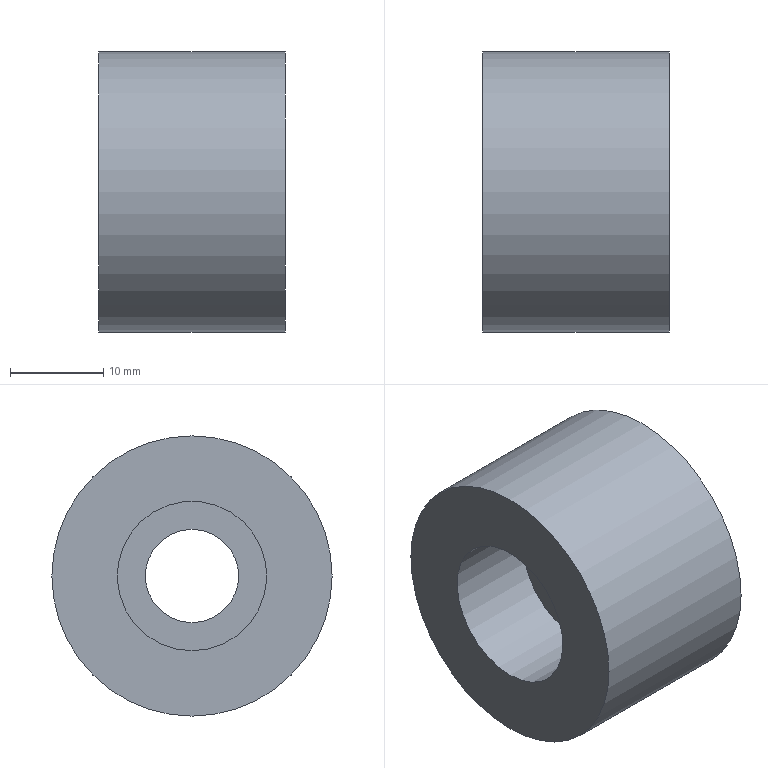Part | NX | features solid 2 | 1 solid | 6 faces | box 20 x 30 x 30 mm | volume 11341 mm3 | cylinder 3 | plane 3 | commonest cylinder face diameters 10 x1 16 x1 30 x1
STEP:
#1=CARTESIAN_POINT('',(-1155.,395.,-130.));
#2=VERTEX_POINT('',#1);
#3=CARTESIAN_POINT('',(-1155.,395.,-115.));
#4=DIRECTION('',(1.,0.,0.));
#5=DIRECTION('',(0.,0.,-1.));
#6=AXIS2_PLACEMENT_3D('',#3,#4,#5);
#7=CIRCLE('',#6,15.);
#8=EDGE_CURVE('',#2,#2,#7,.T.);
#9=ORIENTED_EDGE('',*,*,#8,.F.);
#10=EDGE_LOOP('',(#9));
#11=FACE_BOUND('',#10,.T.);
#12=CARTESIAN_POINT('',(-1175.,395.,-130.));
#13=VERTEX_POINT('',#12);
#14=CARTESIAN_POINT('',(-1175.,395.,-115.));
#15=DIRECTION('',(1.,0.,0.));
#16=DIRECTION('',(0.,0.,-1.));
#17=AXIS2_PLACEMENT_3D('',#14,#15,#16);
#18=CIRCLE('',#17,15.);
#19=EDGE_CURVE('',#13,#13,#18,.T.);
#20=ORIENTED_EDGE('',*,*,#19,.T.);
#21=EDGE_LOOP('',(#20));
#22=FACE_BOUND('',#21,.T.);
#23=CARTESIAN_POINT('',(-1145.,395.,-115.));
#24=DIRECTION('',(-1.,0.,0.));
#25=DIRECTION('',(0.,0.,1.));
#26=AXIS2_PLACEMENT_3D('',#23,#24,#25);
#27=CYLINDRICAL_SURFACE('',#26,15.);
#28=ADVANCED_FACE('',(#11,#22),#27,.T.);
#29=CARTESIAN_POINT('',(-1155.,395.,-120.));
#30=VERTEX_POINT('',#29);
#31=CARTESIAN_POINT('',(-1155.,395.,-115.));
#32=DIRECTION('',(1.,0.,0.));
#33=DIRECTION('',(0.,0.,-1.));
#34=AXIS2_PLACEMENT_3D('',#31,#32,#33);
#35=CIRCLE('',#34,5.);
#36=EDGE_CURVE('',#30,#30,#35,.T.);
#37=ORIENTED_EDGE('',*,*,#36,.F.);
#38=EDGE_LOOP('',(#37));
#39=FACE_BOUND('',#38,.T.);
#40=ORIENTED_EDGE('',*,*,#8,.T.);
#41=EDGE_LOOP('',(#40));
#42=FACE_BOUND('',#41,.T.);
#43=CARTESIAN_POINT('',(-1155.,395.,-115.));
#44=DIRECTION('',(1.,0.,0.));
#45=DIRECTION('',(0.,0.,-1.));
#46=AXIS2_PLACEMENT_3D('',#43,#44,#45);
#47=PLANE('',#46);
#48=ADVANCED_FACE('',(#39,#42),#47,.T.);
#49=CARTESIAN_POINT('',(-1175.,395.,-123.));
#50=VERTEX_POINT('',#49);
#51=CARTESIAN_POINT('',(-1175.,395.,-115.));
#52=DIRECTION('',(1.,0.,0.));
#53=DIRECTION('',(0.,0.,-1.));
#54=AXIS2_PLACEMENT_3D('',#51,#52,#53);
#55=CIRCLE('',#54,8.);
#56=EDGE_CURVE('',#50,#50,#55,.T.);
#57=ORIENTED_EDGE('',*,*,#56,.T.);
#58=EDGE_LOOP('',(#57));
#59=FACE_BOUND('',#58,.T.);
#60=ORIENTED_EDGE('',*,*,#19,.F.);
#61=EDGE_LOOP('',(#60));
#62=FACE_BOUND('',#61,.T.);
#63=CARTESIAN_POINT('',(-1175.,395.,-115.));
#64=DIRECTION('',(1.,0.,0.));
#65=DIRECTION('',(0.,0.,-1.));
#66=AXIS2_PLACEMENT_3D('',#63,#64,#65);
#67=PLANE('',#66);
#68=ADVANCED_FACE('',(#59,#62),#67,.F.);
#69=CARTESIAN_POINT('',(-1165.,395.,-120.));
#70=VERTEX_POINT('',#69);
#71=CARTESIAN_POINT('',(-1165.,395.,-115.));
#72=DIRECTION('',(1.,0.,0.));
#73=DIRECTION('',(0.,0.,-1.));
#74=AXIS2_PLACEMENT_3D('',#71,#72,#73);
#75=CIRCLE('',#74,5.);
#76=EDGE_CURVE('',#70,#70,#75,.T.);
#77=ORIENTED_EDGE('',*,*,#76,.T.);
#78=EDGE_LOOP('',(#77));
#79=FACE_BOUND('',#78,.T.);
#80=CARTESIAN_POINT('',(-1165.,395.,-123.));
#81=VERTEX_POINT('',#80);
#82=CARTESIAN_POINT('',(-1165.,395.,-115.));
#83=DIRECTION('',(1.,0.,0.));
#84=DIRECTION('',(0.,0.,-1.));
#85=AXIS2_PLACEMENT_3D('',#82,#83,#84);
#86=CIRCLE('',#85,8.);
#87=EDGE_CURVE('',#81,#81,#86,.T.);
#88=ORIENTED_EDGE('',*,*,#87,.F.);
#89=EDGE_LOOP('',(#88));
#90=FACE_BOUND('',#89,.T.);
#91=CARTESIAN_POINT('',(-1165.,395.,-115.));
#92=DIRECTION('',(1.,0.,0.));
#93=DIRECTION('',(0.,0.,-1.));
#94=AXIS2_PLACEMENT_3D('',#91,#92,#93);
#95=PLANE('',#94);
#96=ADVANCED_FACE('',(#79,#90),#95,.F.);
#97=ORIENTED_EDGE('',*,*,#87,.T.);
#98=EDGE_LOOP('',(#97));
#99=FACE_BOUND('',#98,.T.);
#100=ORIENTED_EDGE('',*,*,#56,.F.);
#101=EDGE_LOOP('',(#100));
#102=FACE_BOUND('',#101,.T.);
#103=CARTESIAN_POINT('',(-1175.,395.,-115.));
#104=DIRECTION('',(1.,0.,0.));
#105=DIRECTION('',(0.,0.,-1.));
#106=AXIS2_PLACEMENT_3D('',#103,#104,#105);
#107=CYLINDRICAL_SURFACE('',#106,8.);
#108=ADVANCED_FACE('',(#99,#102),#107,.F.);
#109=ORIENTED_EDGE('',*,*,#36,.T.);
#110=EDGE_LOOP('',(#109));
#111=FACE_BOUND('',#110,.T.);
#112=ORIENTED_EDGE('',*,*,#76,.F.);
#113=EDGE_LOOP('',(#112));
#114=FACE_BOUND('',#113,.T.);
#115=CARTESIAN_POINT('',(-1165.,395.,-115.));
#116=DIRECTION('',(1.,0.,0.));
#117=DIRECTION('',(0.,0.,-1.));
#118=AXIS2_PLACEMENT_3D('',#115,#116,#117);
#119=CYLINDRICAL_SURFACE('',#118,5.);
#120=ADVANCED_FACE('',(#111,#114),#119,.F.);
#121=CLOSED_SHELL('',(#28,#48,#68,#96,#108,#120));
#122=MANIFOLD_SOLID_BREP('',#121);
#123=(LENGTH_UNIT()NAMED_UNIT(*)SI_UNIT(.MILLI.,.METRE.));
#124=UNCERTAINTY_MEASURE_WITH_UNIT(LENGTH_MEASURE(0.00001),#123,'','');
#125=(NAMED_UNIT(*)PLANE_ANGLE_UNIT()SI_UNIT($,.RADIAN.));
#126=(NAMED_UNIT(*)SI_UNIT($,.STERADIAN.)SOLID_ANGLE_UNIT());
#127=(GEOMETRIC_REPRESENTATION_CONTEXT(3)GLOBAL_UNCERTAINTY_ASSIGNED_CONTEXT((#124))GLOBAL_UNIT_ASSIGNED_CONTEXT((#123,#125,#126))REPRESENTATION_CONTEXT('',''));
#128=ADVANCED_BREP_SHAPE_REPRESENTATION('',(#122),#127);